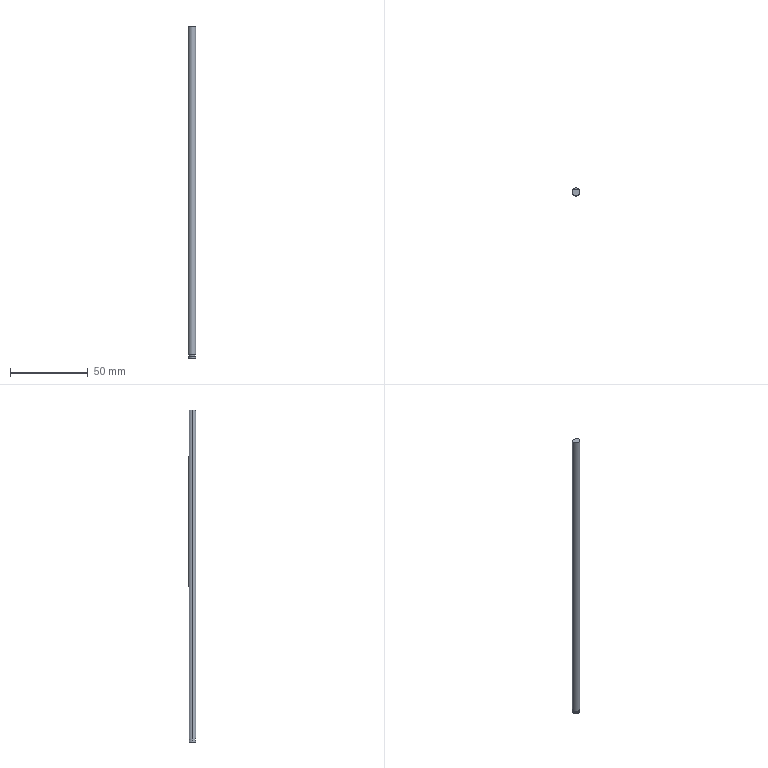Part | SolidWorks | features ICE 3, Extrusion 1 | 1 solid | 16 faces | box 5 x 5 x 213 mm | volume 3913 mm3 | cylinder 8 | plane 8 | commonest cylinder face diameters 5 x5 4 x3
STEP:
#1=CARTESIAN_POINT('',(-2.,0.,1.));
#2=VERTEX_POINT('',#1);
#3=CARTESIAN_POINT('',(-1.054,1.7,1.));
#4=VERTEX_POINT('',#3);
#5=CARTESIAN_POINT('',(0.,0.,1.));
#6=DIRECTION('',(0.,0.,-1.));
#7=DIRECTION('',(-1.,0.,0.));
#8=AXIS2_PLACEMENT_3D('',#5,#6,#7);
#9=CIRCLE('',#8,2.);
#10=EDGE_CURVE('',#2,#4,#9,.T.);
#11=ORIENTED_EDGE('',*,*,#10,.F.);
#12=CARTESIAN_POINT('',(-2.,0.,2.));
#13=VERTEX_POINT('',#12);
#14=CARTESIAN_POINT('',(-2.,0.,1.));
#15=DIRECTION('',(0.,0.,1.));
#16=VECTOR('',#15,1000.);
#17=LINE('',#14,#16);
#18=EDGE_CURVE('',#2,#13,#17,.T.);
#19=ORIENTED_EDGE('',*,*,#18,.T.);
#20=CARTESIAN_POINT('',(-1.054,1.7,2.));
#21=VERTEX_POINT('',#20);
#22=CARTESIAN_POINT('',(0.,0.,2.));
#23=DIRECTION('',(0.,0.,-1.));
#24=DIRECTION('',(-1.,0.,0.));
#25=AXIS2_PLACEMENT_3D('',#22,#23,#24);
#26=CIRCLE('',#25,2.);
#27=EDGE_CURVE('',#13,#21,#26,.T.);
#28=ORIENTED_EDGE('',*,*,#27,.T.);
#29=CARTESIAN_POINT('',(-1.054,1.7,1.));
#30=DIRECTION('',(0.,0.,1.));
#31=VECTOR('',#30,1000.);
#32=LINE('',#29,#31);
#33=EDGE_CURVE('',#4,#21,#32,.T.);
#34=ORIENTED_EDGE('',*,*,#33,.F.);
#35=EDGE_LOOP('',(#11,#19,#28,#34));
#36=FACE_OUTER_BOUND('',#35,.T.);
#37=CARTESIAN_POINT('',(0.,0.,1.));
#38=DIRECTION('',(0.,0.,1.));
#39=DIRECTION('',(1.,0.,0.));
#40=AXIS2_PLACEMENT_3D('',#37,#38,#39);
#41=CYLINDRICAL_SURFACE('',#40,2.);
#42=ADVANCED_FACE('',(#36),#41,.T.);
#43=ORIENTED_EDGE('',*,*,#18,.F.);
#44=CARTESIAN_POINT('',(2.,0.,1.));
#45=VERTEX_POINT('',#44);
#46=CARTESIAN_POINT('',(0.,0.,1.));
#47=DIRECTION('',(0.,0.,-1.));
#48=DIRECTION('',(-1.,0.,0.));
#49=AXIS2_PLACEMENT_3D('',#46,#47,#48);
#50=CIRCLE('',#49,2.);
#51=EDGE_CURVE('',#45,#2,#50,.T.);
#52=ORIENTED_EDGE('',*,*,#51,.F.);
#53=CARTESIAN_POINT('',(2.,0.,2.));
#54=VERTEX_POINT('',#53);
#55=CARTESIAN_POINT('',(2.,0.,1.));
#56=DIRECTION('',(0.,0.,1.));
#57=VECTOR('',#56,1000.);
#58=LINE('',#55,#57);
#59=EDGE_CURVE('',#45,#54,#58,.T.);
#60=ORIENTED_EDGE('',*,*,#59,.T.);
#61=CARTESIAN_POINT('',(0.,0.,2.));
#62=DIRECTION('',(0.,0.,-1.));
#63=DIRECTION('',(-1.,0.,0.));
#64=AXIS2_PLACEMENT_3D('',#61,#62,#63);
#65=CIRCLE('',#64,2.);
#66=EDGE_CURVE('',#54,#13,#65,.T.);
#67=ORIENTED_EDGE('',*,*,#66,.T.);
#68=EDGE_LOOP('',(#43,#52,#60,#67));
#69=FACE_OUTER_BOUND('',#68,.T.);
#70=CARTESIAN_POINT('',(0.,0.,1.));
#71=DIRECTION('',(0.,0.,1.));
#72=DIRECTION('',(1.,0.,0.));
#73=AXIS2_PLACEMENT_3D('',#70,#71,#72);
#74=CYLINDRICAL_SURFACE('',#73,2.);
#75=ADVANCED_FACE('',(#69),#74,.T.);
#76=CARTESIAN_POINT('',(1.833,1.7,1.));
#77=VERTEX_POINT('',#76);
#78=CARTESIAN_POINT('',(2.5,0.,1.));
#79=VERTEX_POINT('',#78);
#80=CARTESIAN_POINT('',(0.,0.,1.));
#81=DIRECTION('',(0.,0.,-1.));
#82=DIRECTION('',(-1.,0.,0.));
#83=AXIS2_PLACEMENT_3D('',#80,#81,#82);
#84=CIRCLE('',#83,2.5);
#85=EDGE_CURVE('',#77,#79,#84,.T.);
#86=ORIENTED_EDGE('',*,*,#85,.T.);
#87=CARTESIAN_POINT('',(2.5,0.,0.));
#88=VERTEX_POINT('',#87);
#89=CARTESIAN_POINT('',(2.5,0.,213.));
#90=DIRECTION('',(0.,0.,-1.));
#91=VECTOR('',#90,1000.);
#92=LINE('',#89,#91);
#93=EDGE_CURVE('',#79,#88,#92,.T.);
#94=ORIENTED_EDGE('',*,*,#93,.T.);
#95=CARTESIAN_POINT('',(1.833,1.7,0.));
#96=VERTEX_POINT('',#95);
#97=CARTESIAN_POINT('',(0.,0.,0.));
#98=DIRECTION('',(0.,0.,1.));
#99=DIRECTION('',(1.,0.,0.));
#100=AXIS2_PLACEMENT_3D('',#97,#98,#99);
#101=CIRCLE('',#100,2.5);
#102=EDGE_CURVE('',#88,#96,#101,.T.);
#103=ORIENTED_EDGE('',*,*,#102,.T.);
#104=CARTESIAN_POINT('',(1.833,1.7,100.));
#105=DIRECTION('',(0.,0.,-1.));
#106=VECTOR('',#105,1000.);
#107=LINE('',#104,#106);
#108=EDGE_CURVE('',#77,#96,#107,.T.);
#109=ORIENTED_EDGE('',*,*,#108,.F.);
#110=EDGE_LOOP('',(#86,#94,#103,#109));
#111=FACE_OUTER_BOUND('',#110,.T.);
#112=CARTESIAN_POINT('',(0.,0.,213.));
#113=DIRECTION('',(0.,0.,-1.));
#114=DIRECTION('',(-1.,0.,0.));
#115=AXIS2_PLACEMENT_3D('',#112,#113,#114);
#116=CYLINDRICAL_SURFACE('',#115,2.5);
#117=ADVANCED_FACE('',(#111),#116,.T.);
#118=ORIENTED_EDGE('',*,*,#93,.F.);
#119=CARTESIAN_POINT('',(-2.5,0.,1.));
#120=VERTEX_POINT('',#119);
#121=CARTESIAN_POINT('',(0.,0.,1.));
#122=DIRECTION('',(0.,0.,-1.));
#123=DIRECTION('',(-1.,0.,0.));
#124=AXIS2_PLACEMENT_3D('',#121,#122,#123);
#125=CIRCLE('',#124,2.5);
#126=EDGE_CURVE('',#79,#120,#125,.T.);
#127=ORIENTED_EDGE('',*,*,#126,.T.);
#128=CARTESIAN_POINT('',(-2.5,0.,0.));
#129=VERTEX_POINT('',#128);
#130=CARTESIAN_POINT('',(-2.5,0.,213.));
#131=DIRECTION('',(0.,0.,-1.));
#132=VECTOR('',#131,1000.);
#133=LINE('',#130,#132);
#134=EDGE_CURVE('',#120,#129,#133,.T.);
#135=ORIENTED_EDGE('',*,*,#134,.T.);
#136=CARTESIAN_POINT('',(0.,0.,0.));
#137=DIRECTION('',(0.,0.,1.));
#138=DIRECTION('',(1.,0.,0.));
#139=AXIS2_PLACEMENT_3D('',#136,#137,#138);
#140=CIRCLE('',#139,2.5);
#141=EDGE_CURVE('',#129,#88,#140,.T.);
#142=ORIENTED_EDGE('',*,*,#141,.T.);
#143=EDGE_LOOP('',(#118,#127,#135,#142));
#144=FACE_OUTER_BOUND('',#143,.T.);
#145=CARTESIAN_POINT('',(0.,0.,213.));
#146=DIRECTION('',(0.,0.,-1.));
#147=DIRECTION('',(-1.,0.,0.));
#148=AXIS2_PLACEMENT_3D('',#145,#146,#147);
#149=CYLINDRICAL_SURFACE('',#148,2.5);
#150=ADVANCED_FACE('',(#144),#149,.T.);
#151=CARTESIAN_POINT('',(2.5,0.,213.));
#152=VERTEX_POINT('',#151);
#153=CARTESIAN_POINT('',(1.835,1.698,213.));
#154=VERTEX_POINT('',#153);
#155=CARTESIAN_POINT('',(0.,0.,213.));
#156=DIRECTION('',(0.,0.,1.));
#157=DIRECTION('',(1.,0.,0.));
#158=AXIS2_PLACEMENT_3D('',#155,#156,#157);
#159=CIRCLE('',#158,2.5);
#160=EDGE_CURVE('',#152,#154,#159,.T.);
#161=ORIENTED_EDGE('',*,*,#160,.F.);
#162=CARTESIAN_POINT('',(2.5,0.,2.));
#163=VERTEX_POINT('',#162);
#164=CARTESIAN_POINT('',(2.5,0.,213.));
#165=DIRECTION('',(0.,0.,-1.));
#166=VECTOR('',#165,1000.);
#167=LINE('',#164,#166);
#168=EDGE_CURVE('',#152,#163,#167,.T.);
#169=ORIENTED_EDGE('',*,*,#168,.T.);
#170=CARTESIAN_POINT('',(1.833,1.7,2.));
#171=VERTEX_POINT('',#170);
#172=CARTESIAN_POINT('',(0.,0.,2.));
#173=DIRECTION('',(0.,0.,-1.));
#174=DIRECTION('',(-1.,0.,0.));
#175=AXIS2_PLACEMENT_3D('',#172,#173,#174);
#176=CIRCLE('',#175,2.5);
#177=EDGE_CURVE('',#171,#163,#176,.T.);
#178=ORIENTED_EDGE('',*,*,#177,.F.);
#179=CARTESIAN_POINT('',(1.833,1.7,100.));
#180=VERTEX_POINT('',#179);
#181=CARTESIAN_POINT('',(1.833,1.7,100.));
#182=DIRECTION('',(0.,0.,-1.));
#183=VECTOR('',#182,1000.);
#184=LINE('',#181,#183);
#185=EDGE_CURVE('',#180,#171,#184,.T.);
#186=ORIENTED_EDGE('',*,*,#185,.F.);
#187=CARTESIAN_POINT('',(-1.833,1.7,100.));
#188=VERTEX_POINT('',#187);
#189=CARTESIAN_POINT('',(0.,0.,100.));
#190=DIRECTION('',(0.,0.,-1.));
#191=DIRECTION('',(-1.,0.,0.));
#192=AXIS2_PLACEMENT_3D('',#189,#190,#191);
#193=CIRCLE('',#192,2.5);
#194=EDGE_CURVE('',#188,#180,#193,.T.);
#195=ORIENTED_EDGE('',*,*,#194,.F.);
#196=CARTESIAN_POINT('',(-1.833,1.7,2.));
#197=VERTEX_POINT('',#196);
#198=CARTESIAN_POINT('',(-1.833,1.7,100.));
#199=DIRECTION('',(0.,0.,-1.));
#200=VECTOR('',#199,1000.);
#201=LINE('',#198,#200);
#202=EDGE_CURVE('',#188,#197,#201,.T.);
#203=ORIENTED_EDGE('',*,*,#202,.T.);
#204=CARTESIAN_POINT('',(-2.5,0.,2.));
#205=VERTEX_POINT('',#204);
#206=CARTESIAN_POINT('',(0.,0.,2.));
#207=DIRECTION('',(0.,0.,-1.));
#208=DIRECTION('',(-1.,0.,0.));
#209=AXIS2_PLACEMENT_3D('',#206,#207,#208);
#210=CIRCLE('',#209,2.5);
#211=EDGE_CURVE('',#205,#197,#210,.T.);
#212=ORIENTED_EDGE('',*,*,#211,.F.);
#213=CARTESIAN_POINT('',(-2.5,0.,213.));
#214=VERTEX_POINT('',#213);
#215=CARTESIAN_POINT('',(-2.5,0.,213.));
#216=DIRECTION('',(0.,0.,-1.));
#217=VECTOR('',#216,1000.);
#218=LINE('',#215,#217);
#219=EDGE_CURVE('',#214,#205,#218,.T.);
#220=ORIENTED_EDGE('',*,*,#219,.F.);
#221=CARTESIAN_POINT('',(-1.835,1.698,213.));
#222=VERTEX_POINT('',#221);
#223=CARTESIAN_POINT('',(0.,0.,213.));
#224=DIRECTION('',(0.,0.,1.));
#225=DIRECTION('',(1.,0.,0.));
#226=AXIS2_PLACEMENT_3D('',#223,#224,#225);
#227=CIRCLE('',#226,2.5);
#228=EDGE_CURVE('',#222,#214,#227,.T.);
#229=ORIENTED_EDGE('',*,*,#228,.F.);
#230=CARTESIAN_POINT('',(-1.835,1.698,183.));
#231=VERTEX_POINT('',#230);
#232=CARTESIAN_POINT('',(-1.835,1.698,183.));
#233=DIRECTION('',(0.,0.,1.));
#234=VECTOR('',#233,1000.);
#235=LINE('',#232,#234);
#236=EDGE_CURVE('',#231,#222,#235,.T.);
#237=ORIENTED_EDGE('',*,*,#236,.F.);
#238=CARTESIAN_POINT('',(1.835,1.698,183.));
#239=VERTEX_POINT('',#238);
#240=CARTESIAN_POINT('',(0.,0.,183.));
#241=DIRECTION('',(0.,0.,1.));
#242=DIRECTION('',(1.,0.,0.));
#243=AXIS2_PLACEMENT_3D('',#240,#241,#242);
#244=CIRCLE('',#243,2.5);
#245=EDGE_CURVE('',#239,#231,#244,.T.);
#246=ORIENTED_EDGE('',*,*,#245,.F.);
#247=CARTESIAN_POINT('',(1.835,1.698,183.));
#248=DIRECTION('',(0.,0.,1.));
#249=VECTOR('',#248,1000.);
#250=LINE('',#247,#249);
#251=EDGE_CURVE('',#239,#154,#250,.T.);
#252=ORIENTED_EDGE('',*,*,#251,.T.);
#253=EDGE_LOOP('',(#161,#169,#178,#186,#195,#203,#212,#220,#229,#237,#246,#252));
#254=FACE_OUTER_BOUND('',#253,.T.);
#255=CARTESIAN_POINT('',(0.,0.,213.));
#256=DIRECTION('',(0.,0.,-1.));
#257=DIRECTION('',(-1.,0.,0.));
#258=AXIS2_PLACEMENT_3D('',#255,#256,#257);
#259=CYLINDRICAL_SURFACE('',#258,2.5);
#260=ADVANCED_FACE('',(#254),#259,.T.);
#261=ORIENTED_EDGE('',*,*,#168,.F.);
#262=CARTESIAN_POINT('',(0.,0.,213.));
#263=DIRECTION('',(0.,0.,1.));
#264=DIRECTION('',(1.,0.,0.));
#265=AXIS2_PLACEMENT_3D('',#262,#263,#264);
#266=CIRCLE('',#265,2.5);
#267=EDGE_CURVE('',#214,#152,#266,.T.);
#268=ORIENTED_EDGE('',*,*,#267,.F.);
#269=ORIENTED_EDGE('',*,*,#219,.T.);
#270=CARTESIAN_POINT('',(0.,0.,2.));
#271=DIRECTION('',(0.,0.,-1.));
#272=DIRECTION('',(-1.,0.,0.));
#273=AXIS2_PLACEMENT_3D('',#270,#271,#272);
#274=CIRCLE('',#273,2.5);
#275=EDGE_CURVE('',#163,#205,#274,.T.);
#276=ORIENTED_EDGE('',*,*,#275,.F.);
#277=EDGE_LOOP('',(#261,#268,#269,#276));
#278=FACE_OUTER_BOUND('',#277,.T.);
#279=CARTESIAN_POINT('',(0.,0.,213.));
#280=DIRECTION('',(0.,0.,-1.));
#281=DIRECTION('',(-1.,0.,0.));
#282=AXIS2_PLACEMENT_3D('',#279,#280,#281);
#283=CYLINDRICAL_SURFACE('',#282,2.5);
#284=ADVANCED_FACE('',(#278),#283,.T.);
#285=ORIENTED_EDGE('',*,*,#134,.F.);
#286=CARTESIAN_POINT('',(-1.833,1.7,1.));
#287=VERTEX_POINT('',#286);
#288=CARTESIAN_POINT('',(0.,0.,1.));
#289=DIRECTION('',(0.,0.,-1.));
#290=DIRECTION('',(-1.,0.,0.));
#291=AXIS2_PLACEMENT_3D('',#288,#289,#290);
#292=CIRCLE('',#291,2.5);
#293=EDGE_CURVE('',#120,#287,#292,.T.);
#294=ORIENTED_EDGE('',*,*,#293,.T.);
#295=CARTESIAN_POINT('',(-1.833,1.7,0.));
#296=VERTEX_POINT('',#295);
#297=CARTESIAN_POINT('',(-1.833,1.7,100.));
#298=DIRECTION('',(0.,0.,-1.));
#299=VECTOR('',#298,1000.);
#300=LINE('',#297,#299);
#301=EDGE_CURVE('',#287,#296,#300,.T.);
#302=ORIENTED_EDGE('',*,*,#301,.T.);
#303=CARTESIAN_POINT('',(0.,0.,0.));
#304=DIRECTION('',(0.,0.,1.));
#305=DIRECTION('',(1.,0.,0.));
#306=AXIS2_PLACEMENT_3D('',#303,#304,#305);
#307=CIRCLE('',#306,2.5);
#308=EDGE_CURVE('',#296,#129,#307,.T.);
#309=ORIENTED_EDGE('',*,*,#308,.T.);
#310=EDGE_LOOP('',(#285,#294,#302,#309));
#311=FACE_OUTER_BOUND('',#310,.T.);
#312=CARTESIAN_POINT('',(0.,0.,213.));
#313=DIRECTION('',(0.,0.,-1.));
#314=DIRECTION('',(-1.,0.,0.));
#315=AXIS2_PLACEMENT_3D('',#312,#313,#314);
#316=CYLINDRICAL_SURFACE('',#315,2.5);
#317=ADVANCED_FACE('',(#311),#316,.T.);
#318=CARTESIAN_POINT('',(-1.835,1.698,213.));
#319=DIRECTION('',(1.,0.,0.));
#320=VECTOR('',#319,1000.);
#321=LINE('',#318,#320);
#322=EDGE_CURVE('',#222,#154,#321,.T.);
#323=ORIENTED_EDGE('',*,*,#322,.F.);
#324=ORIENTED_EDGE('',*,*,#228,.T.);
#325=ORIENTED_EDGE('',*,*,#267,.T.);
#326=ORIENTED_EDGE('',*,*,#160,.T.);
#327=EDGE_LOOP('',(#323,#324,#325,#326));
#328=FACE_OUTER_BOUND('',#327,.T.);
#329=CARTESIAN_POINT('',(0.,0.,213.));
#330=DIRECTION('',(0.,0.,1.));
#331=DIRECTION('',(1.,0.,0.));
#332=AXIS2_PLACEMENT_3D('',#329,#330,#331);
#333=PLANE('',#332);
#334=ADVANCED_FACE('',(#328),#333,.T.);
#335=ORIENTED_EDGE('',*,*,#308,.F.);
#336=CARTESIAN_POINT('',(1.833,1.7,0.));
#337=DIRECTION('',(-1.,0.,0.));
#338=VECTOR('',#337,1000.);
#339=LINE('',#336,#338);
#340=EDGE_CURVE('',#96,#296,#339,.T.);
#341=ORIENTED_EDGE('',*,*,#340,.F.);
#342=ORIENTED_EDGE('',*,*,#102,.F.);
#343=ORIENTED_EDGE('',*,*,#141,.F.);
#344=EDGE_LOOP('',(#335,#341,#342,#343));
#345=FACE_OUTER_BOUND('',#344,.T.);
#346=CARTESIAN_POINT('',(0.,0.,0.));
#347=DIRECTION('',(0.,0.,1.));
#348=DIRECTION('',(1.,0.,0.));
#349=AXIS2_PLACEMENT_3D('',#346,#347,#348);
#350=PLANE('',#349);
#351=ADVANCED_FACE('',(#345),#350,.F.);
#352=CARTESIAN_POINT('',(1.054,1.7,2.));
#353=VERTEX_POINT('',#352);
#354=CARTESIAN_POINT('',(1.054,1.7,1.));
#355=VERTEX_POINT('',#354);
#356=CARTESIAN_POINT('',(1.054,1.7,1.));
#357=DIRECTION('',(0.,0.,-1.));
#358=VECTOR('',#357,1000.);
#359=LINE('',#356,#358);
#360=EDGE_CURVE('',#353,#355,#359,.T.);
#361=ORIENTED_EDGE('',*,*,#360,.T.);
#362=CARTESIAN_POINT('',(1.833,1.7,1.));
#363=DIRECTION('',(1.,0.,0.));
#364=VECTOR('',#363,1000.);
#365=LINE('',#362,#364);
#366=EDGE_CURVE('',#355,#77,#365,.T.);
#367=ORIENTED_EDGE('',*,*,#366,.T.);
#368=ORIENTED_EDGE('',*,*,#108,.T.);
#369=ORIENTED_EDGE('',*,*,#340,.T.);
#370=ORIENTED_EDGE('',*,*,#301,.F.);
#371=CARTESIAN_POINT('',(1.833,1.7,1.));
#372=DIRECTION('',(1.,0.,0.));
#373=VECTOR('',#372,1000.);
#374=LINE('',#371,#373);
#375=EDGE_CURVE('',#287,#4,#374,.T.);
#376=ORIENTED_EDGE('',*,*,#375,.T.);
#377=ORIENTED_EDGE('',*,*,#33,.T.);
#378=CARTESIAN_POINT('',(1.833,1.7,2.));
#379=DIRECTION('',(1.,0.,0.));
#380=VECTOR('',#379,1000.);
#381=LINE('',#378,#380);
#382=EDGE_CURVE('',#197,#21,#381,.T.);
#383=ORIENTED_EDGE('',*,*,#382,.F.);
#384=ORIENTED_EDGE('',*,*,#202,.F.);
#385=CARTESIAN_POINT('',(1.833,1.7,100.));
#386=DIRECTION('',(-1.,0.,0.));
#387=VECTOR('',#386,1000.);
#388=LINE('',#385,#387);
#389=EDGE_CURVE('',#180,#188,#388,.T.);
#390=ORIENTED_EDGE('',*,*,#389,.F.);
#391=ORIENTED_EDGE('',*,*,#185,.T.);
#392=CARTESIAN_POINT('',(1.833,1.7,2.));
#393=DIRECTION('',(1.,0.,0.));
#394=VECTOR('',#393,1000.);
#395=LINE('',#392,#394);
#396=EDGE_CURVE('',#353,#171,#395,.T.);
#397=ORIENTED_EDGE('',*,*,#396,.F.);
#398=EDGE_LOOP('',(#361,#367,#368,#369,#370,#376,#377,#383,#384,#390,#391,#397));
#399=FACE_OUTER_BOUND('',#398,.T.);
#400=CARTESIAN_POINT('',(1.833,1.7,100.));
#401=DIRECTION('',(0.,-1.,0.));
#402=DIRECTION('',(0.,0.,-1.));
#403=AXIS2_PLACEMENT_3D('',#400,#401,#402);
#404=PLANE('',#403);
#405=ADVANCED_FACE('',(#399),#404,.F.);
#406=ORIENTED_EDGE('',*,*,#194,.T.);
#407=ORIENTED_EDGE('',*,*,#389,.T.);
#408=EDGE_LOOP('',(#406,#407));
#409=FACE_OUTER_BOUND('',#408,.T.);
#410=CARTESIAN_POINT('',(0.,0.,100.));
#411=DIRECTION('',(0.,0.,-1.));
#412=DIRECTION('',(-1.,0.,0.));
#413=AXIS2_PLACEMENT_3D('',#410,#411,#412);
#414=PLANE('',#413);
#415=ADVANCED_FACE('',(#409),#414,.T.);
#416=ORIENTED_EDGE('',*,*,#85,.F.);
#417=ORIENTED_EDGE('',*,*,#366,.F.);
#418=CARTESIAN_POINT('',(0.,0.,1.));
#419=DIRECTION('',(0.,0.,-1.));
#420=DIRECTION('',(-1.,0.,0.));
#421=AXIS2_PLACEMENT_3D('',#418,#419,#420);
#422=CIRCLE('',#421,2.);
#423=EDGE_CURVE('',#355,#45,#422,.T.);
#424=ORIENTED_EDGE('',*,*,#423,.T.);
#425=ORIENTED_EDGE('',*,*,#51,.T.);
#426=ORIENTED_EDGE('',*,*,#10,.T.);
#427=ORIENTED_EDGE('',*,*,#375,.F.);
#428=ORIENTED_EDGE('',*,*,#293,.F.);
#429=ORIENTED_EDGE('',*,*,#126,.F.);
#430=EDGE_LOOP('',(#416,#417,#424,#425,#426,#427,#428,#429));
#431=FACE_OUTER_BOUND('',#430,.T.);
#432=CARTESIAN_POINT('',(0.,0.,1.));
#433=DIRECTION('',(0.,0.,-1.));
#434=DIRECTION('',(-1.,0.,0.));
#435=AXIS2_PLACEMENT_3D('',#432,#433,#434);
#436=PLANE('',#435);
#437=ADVANCED_FACE('',(#431),#436,.F.);
#438=ORIENTED_EDGE('',*,*,#382,.T.);
#439=ORIENTED_EDGE('',*,*,#27,.F.);
#440=ORIENTED_EDGE('',*,*,#66,.F.);
#441=CARTESIAN_POINT('',(0.,0.,2.));
#442=DIRECTION('',(0.,0.,-1.));
#443=DIRECTION('',(-1.,0.,0.));
#444=AXIS2_PLACEMENT_3D('',#441,#442,#443);
#445=CIRCLE('',#444,2.);
#446=EDGE_CURVE('',#353,#54,#445,.T.);
#447=ORIENTED_EDGE('',*,*,#446,.F.);
#448=ORIENTED_EDGE('',*,*,#396,.T.);
#449=ORIENTED_EDGE('',*,*,#177,.T.);
#450=ORIENTED_EDGE('',*,*,#275,.T.);
#451=ORIENTED_EDGE('',*,*,#211,.T.);
#452=EDGE_LOOP('',(#438,#439,#440,#447,#448,#449,#450,#451));
#453=FACE_OUTER_BOUND('',#452,.T.);
#454=CARTESIAN_POINT('',(0.,0.,2.));
#455=DIRECTION('',(0.,0.,-1.));
#456=DIRECTION('',(-1.,0.,0.));
#457=AXIS2_PLACEMENT_3D('',#454,#455,#456);
#458=PLANE('',#457);
#459=ADVANCED_FACE('',(#453),#458,.T.);
#460=ORIENTED_EDGE('',*,*,#59,.F.);
#461=ORIENTED_EDGE('',*,*,#423,.F.);
#462=ORIENTED_EDGE('',*,*,#360,.F.);
#463=ORIENTED_EDGE('',*,*,#446,.T.);
#464=EDGE_LOOP('',(#460,#461,#462,#463));
#465=FACE_OUTER_BOUND('',#464,.T.);
#466=CARTESIAN_POINT('',(0.,0.,1.));
#467=DIRECTION('',(0.,0.,1.));
#468=DIRECTION('',(1.,0.,0.));
#469=AXIS2_PLACEMENT_3D('',#466,#467,#468);
#470=CYLINDRICAL_SURFACE('',#469,2.);
#471=ADVANCED_FACE('',(#465),#470,.T.);
#472=ORIENTED_EDGE('',*,*,#322,.T.);
#473=ORIENTED_EDGE('',*,*,#251,.F.);
#474=CARTESIAN_POINT('',(-1.835,1.698,183.));
#475=DIRECTION('',(1.,0.,0.));
#476=VECTOR('',#475,1000.);
#477=LINE('',#474,#476);
#478=EDGE_CURVE('',#231,#239,#477,.T.);
#479=ORIENTED_EDGE('',*,*,#478,.F.);
#480=ORIENTED_EDGE('',*,*,#236,.T.);
#481=EDGE_LOOP('',(#472,#473,#479,#480));
#482=FACE_OUTER_BOUND('',#481,.T.);
#483=CARTESIAN_POINT('',(-1.835,1.698,183.));
#484=DIRECTION('',(0.,-1.,0.));
#485=DIRECTION('',(0.,0.,-1.));
#486=AXIS2_PLACEMENT_3D('',#483,#484,#485);
#487=PLANE('',#486);
#488=ADVANCED_FACE('',(#482),#487,.F.);
#489=ORIENTED_EDGE('',*,*,#245,.T.);
#490=ORIENTED_EDGE('',*,*,#478,.T.);
#491=EDGE_LOOP('',(#489,#490));
#492=FACE_OUTER_BOUND('',#491,.T.);
#493=CARTESIAN_POINT('',(0.,0.,183.));
#494=DIRECTION('',(0.,0.,1.));
#495=DIRECTION('',(1.,0.,0.));
#496=AXIS2_PLACEMENT_3D('',#493,#494,#495);
#497=PLANE('',#496);
#498=ADVANCED_FACE('',(#492),#497,.T.);
#499=CLOSED_SHELL('',(#42,#75,#117,#150,#260,#284,#317,#334,#351,#405,#415,#437,#459,#471,#488,#498));
#500=MANIFOLD_SOLID_BREP('',#499);
#501=CARTESIAN_POINT('',(0.,0.,0.));
#502=DIRECTION('',(0.,0.,1.));
#503=DIRECTION('',(1.,0.,0.));
#504=AXIS2_PLACEMENT_3D('',#501,#502,#503);
#505=(LENGTH_UNIT()NAMED_UNIT(*)SI_UNIT(.MILLI.,.METRE.));
#506=UNCERTAINTY_MEASURE_WITH_UNIT(LENGTH_MEASURE(0.00001),#505,'','');
#507=(NAMED_UNIT(*)PLANE_ANGLE_UNIT()SI_UNIT($,.RADIAN.));
#508=(NAMED_UNIT(*)SI_UNIT($,.STERADIAN.)SOLID_ANGLE_UNIT());
#509=(GEOMETRIC_REPRESENTATION_CONTEXT(3)GLOBAL_UNCERTAINTY_ASSIGNED_CONTEXT((#506))GLOBAL_UNIT_ASSIGNED_CONTEXT((#505,#507,#508))REPRESENTATION_CONTEXT('',''));
#510=ADVANCED_BREP_SHAPE_REPRESENTATION('',(#500,#504),#509);